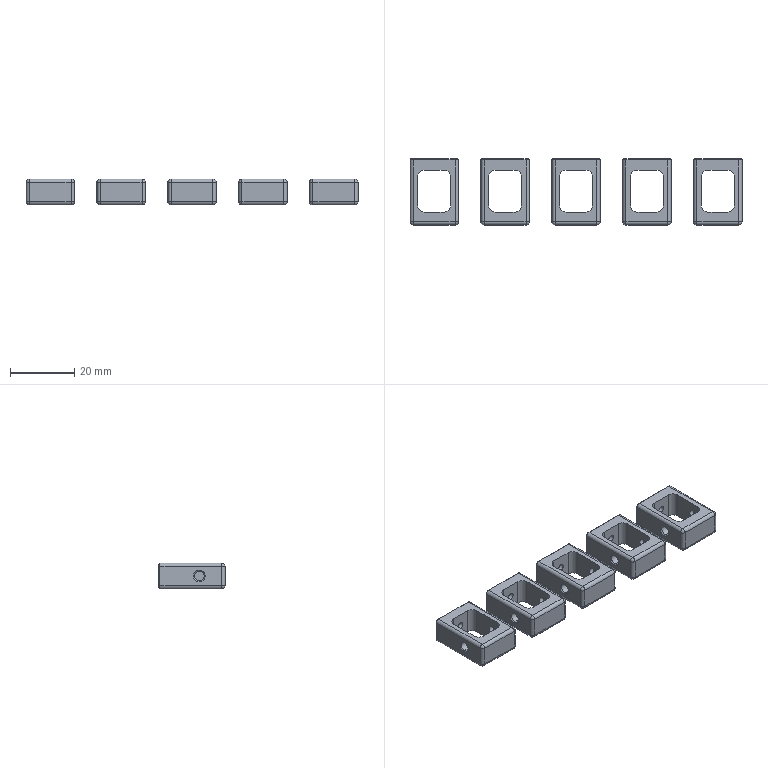NC program | NX | posted with a generic post | part box 103 x 20.5 x 8 mm
Lines 1 to 18 of 9732:
N10 G17 G21 G94 G90
(FLOOR_WALL , TOOL : D80)
N12 T19 M6
N14 G54
N16 G17 G0 G90 X-96.5 Y0. S6500 M3
N18 G43 Z30. H19
N20 Z3.
N22 G94 G1 Z0. F1500.
N24 X-93.5
N26 X93.5
N28 X96.5
N30 Z3.
N32 G0 Z30.
N34 M5